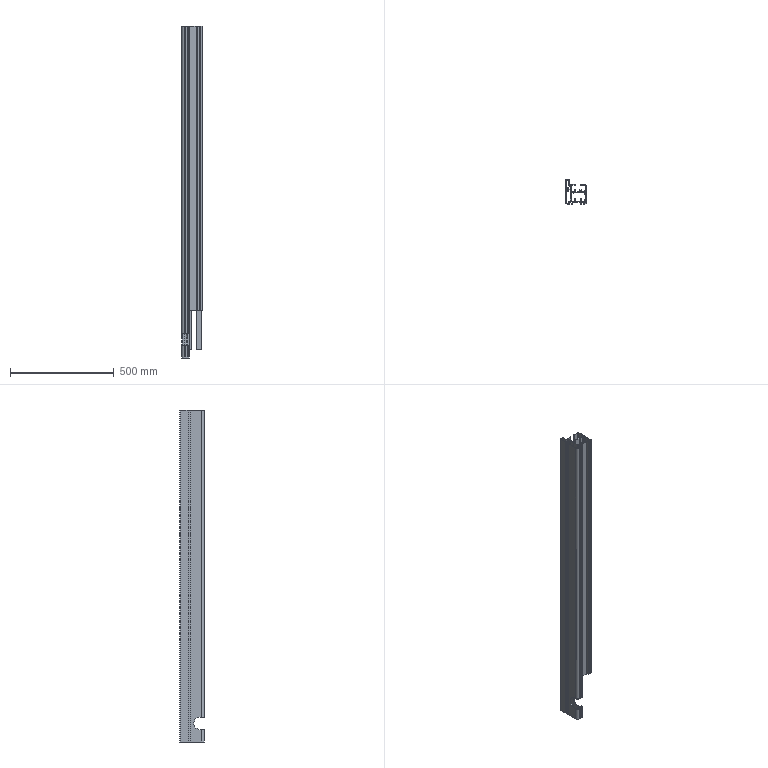Part | STEP file | PN_0009_default | 1 solid | 246 faces | box 100 x 118 x 1600 mm | volume 2644329 mm3 | plane 147 | cylinder 99 | commonest cylinder face diameters 1 x65 4 x24 2 x2 20 x2 24 x2 60 x2